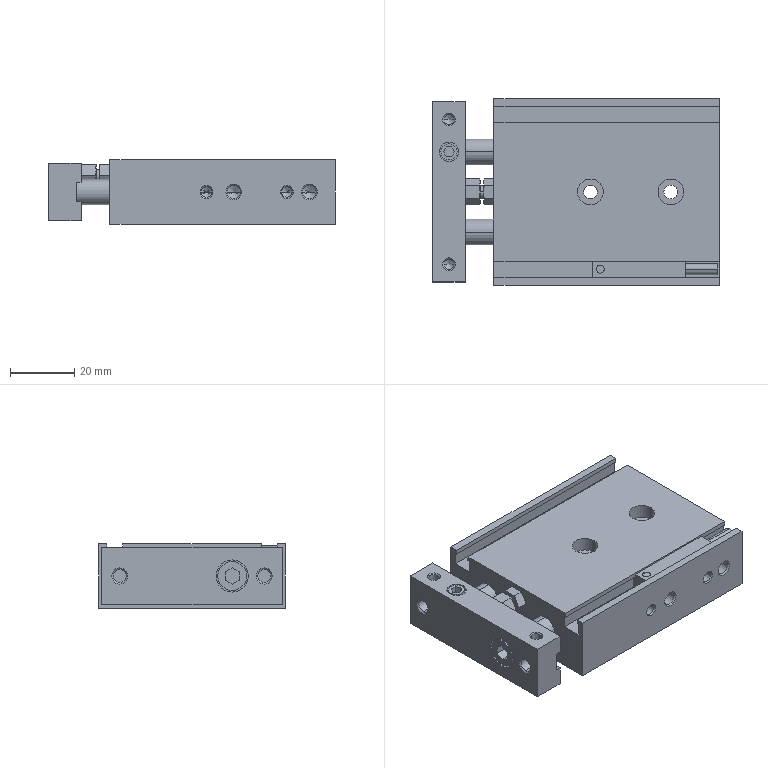Part | SolidWorks | features AEMSimFeature 1 | 3 solids | 243 faces | box 89 x 58 x 20 mm | volume 84198 mm3 | plane 93 | cone 84 | cylinder 66 | commonest cylinder face diameters 3.242 x16 4.134 x12 8 x12 15 x8 4.3 x4 2.5 x2